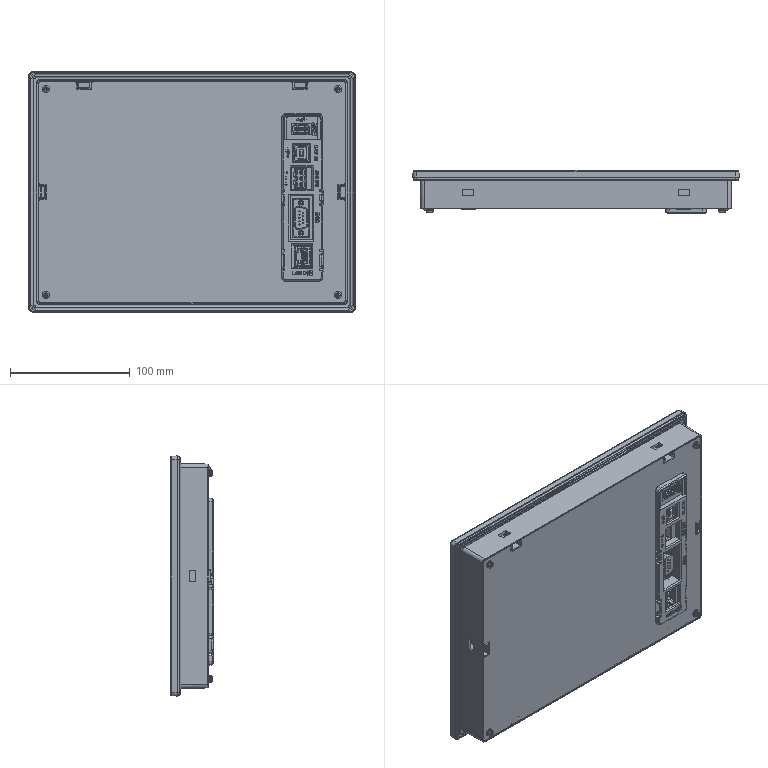Part | SolidWorks | 37 solids | 5085 faces | volume 566898 mm3 | plane 3087 | cylinder 1213 | spline 618 | cone 131 | torus 36 | commonest cylinder face diameters 1 x200 3 x102 2 x95 0.5 x89 0.4 x79 0.6 x66